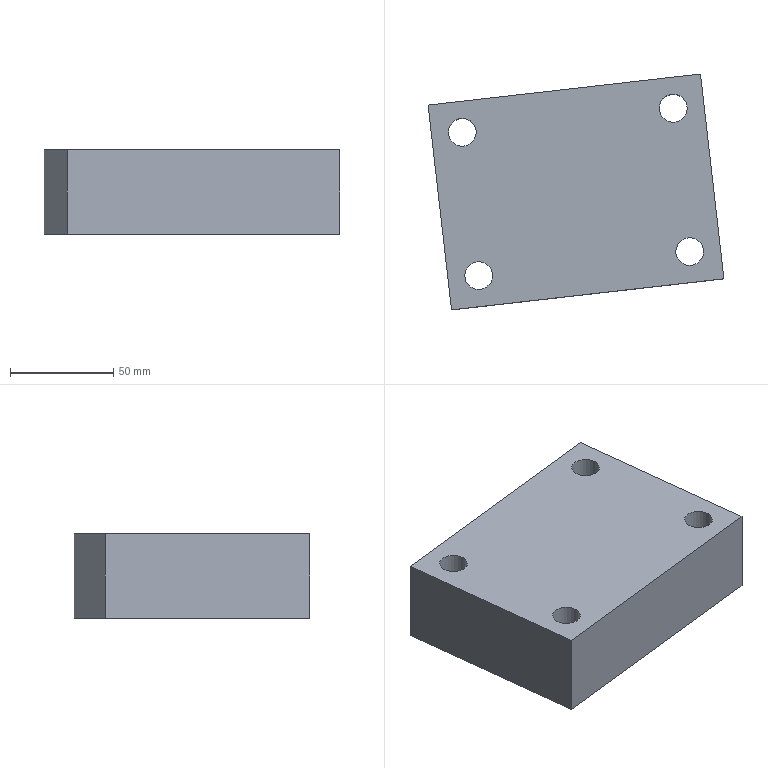Part | NX | features solid 2 | 1 solid | 18 faces | box 143.465 x 114.413 x 41 mm | volume 511564 mm3 | plane 10 | cylinder 8 | commonest cylinder face diameters 13.5 x4 20 x4
STEP:
#1=CARTESIAN_POINT('',(2599.823,120.761,101.));
#2=VERTEX_POINT('',#1);
#3=CARTESIAN_POINT('',(2593.073,120.761,101.));
#4=DIRECTION('',(0.,0.,1.));
#5=DIRECTION('',(1.,0.,0.));
#6=AXIS2_PLACEMENT_3D('',#3,#4,#5);
#7=CIRCLE('',#6,6.75);
#8=EDGE_CURVE('',#2,#2,#7,.T.);
#9=ORIENTED_EDGE('',*,*,#8,.F.);
#10=EDGE_LOOP('',(#9));
#11=FACE_BOUND('',#10,.T.);
#12=CARTESIAN_POINT('',(2607.575,52.73,101.));
#13=VERTEX_POINT('',#12);
#14=CARTESIAN_POINT('',(2600.998,51.211,101.));
#15=DIRECTION('',(0.,0.,-1.));
#16=DIRECTION('',(0.9744,0.225,0.));
#17=AXIS2_PLACEMENT_3D('',#14,#15,#16);
#18=CIRCLE('',#17,6.75);
#19=EDGE_CURVE('',#13,#13,#18,.T.);
#20=ORIENTED_EDGE('',*,*,#19,.T.);
#21=EDGE_LOOP('',(#20));
#22=FACE_BOUND('',#21,.T.);
#23=CARTESIAN_POINT('',(2606.279,137.363,101.));
#24=VERTEX_POINT('',#23);
#25=CARTESIAN_POINT('',(2474.134,122.307,101.));
#26=VERTEX_POINT('',#25);
#27=CARTESIAN_POINT('',(2529.774,128.646,101.));
#28=DIRECTION('',(-0.9936,-0.1132,0.));
#29=VECTOR('',#28,1000.);
#30=LINE('',#27,#29);
#31=EDGE_CURVE('',#24,#26,#30,.T.);
#32=ORIENTED_EDGE('',*,*,#31,.T.);
#33=CARTESIAN_POINT('',(2485.454,22.95,101.));
#34=VERTEX_POINT('',#33);
#35=CARTESIAN_POINT('',(2480.36,67.661,101.));
#36=DIRECTION('',(0.1132,-0.9936,0.));
#37=VECTOR('',#36,1000.);
#38=LINE('',#35,#37);
#39=EDGE_CURVE('',#26,#34,#38,.T.);
#40=ORIENTED_EDGE('',*,*,#39,.T.);
#41=CARTESIAN_POINT('',(2617.599,38.006,101.));
#42=VERTEX_POINT('',#41);
#43=CARTESIAN_POINT('',(2541.094,29.289,101.));
#44=DIRECTION('',(0.9936,0.1132,0.));
#45=VECTOR('',#44,1000.);
#46=LINE('',#43,#45);
#47=EDGE_CURVE('',#34,#42,#46,.T.);
#48=ORIENTED_EDGE('',*,*,#47,.T.);
#49=CARTESIAN_POINT('',(2612.505,82.717,101.));
#50=DIRECTION('',(-0.1132,0.9936,0.));
#51=VECTOR('',#50,1000.);
#52=LINE('',#49,#51);
#53=EDGE_CURVE('',#42,#24,#52,.T.);
#54=ORIENTED_EDGE('',*,*,#53,.T.);
#55=EDGE_LOOP('',(#32,#40,#48,#54));
#56=FACE_BOUND('',#55,.T.);
#57=CARTESIAN_POINT('',(2484.158,107.583,101.));
#58=VERTEX_POINT('',#57);
#59=CARTESIAN_POINT('',(2490.735,109.102,101.));
#60=DIRECTION('',(0.,0.,-1.));
#61=DIRECTION('',(-0.9744,-0.225,0.));
#62=AXIS2_PLACEMENT_3D('',#59,#60,#61);
#63=CIRCLE('',#62,6.75);
#64=EDGE_CURVE('',#58,#58,#63,.T.);
#65=ORIENTED_EDGE('',*,*,#64,.T.);
#66=EDGE_LOOP('',(#65));
#67=FACE_BOUND('',#66,.T.);
#68=CARTESIAN_POINT('',(2491.91,39.552,101.));
#69=VERTEX_POINT('',#68);
#70=CARTESIAN_POINT('',(2498.66,39.552,101.));
#71=DIRECTION('',(0.,0.,1.));
#72=DIRECTION('',(-1.,0.,0.));
#73=AXIS2_PLACEMENT_3D('',#70,#71,#72);
#74=CIRCLE('',#73,6.75);
#75=EDGE_CURVE('',#69,#69,#74,.T.);
#76=ORIENTED_EDGE('',*,*,#75,.F.);
#77=EDGE_LOOP('',(#76));
#78=FACE_BOUND('',#77,.T.);
#79=CARTESIAN_POINT('',(282.5,-193.,101.));
#80=DIRECTION('',(0.,0.,1.));
#81=DIRECTION('',(-1.,0.,0.));
#82=AXIS2_PLACEMENT_3D('',#79,#80,#81);
#83=PLANE('',#82);
#84=ADVANCED_FACE('',(#11,#22,#56,#67,#78),#83,.T.);
#85=CARTESIAN_POINT('',(2603.073,120.761,60.));
#86=VERTEX_POINT('',#85);
#87=CARTESIAN_POINT('',(2593.073,120.761,60.));
#88=DIRECTION('',(0.,0.,-1.));
#89=DIRECTION('',(1.,0.,0.));
#90=AXIS2_PLACEMENT_3D('',#87,#88,#89);
#91=CIRCLE('',#90,10.);
#92=EDGE_CURVE('',#86,#86,#91,.T.);
#93=ORIENTED_EDGE('',*,*,#92,.F.);
#94=EDGE_LOOP('',(#93));
#95=FACE_BOUND('',#94,.T.);
#96=CARTESIAN_POINT('',(2610.741,53.461,60.));
#97=VERTEX_POINT('',#96);
#98=CARTESIAN_POINT('',(2600.998,51.211,60.));
#99=DIRECTION('',(0.,0.,1.));
#100=DIRECTION('',(0.9744,0.225,0.));
#101=AXIS2_PLACEMENT_3D('',#98,#99,#100);
#102=CIRCLE('',#101,10.);
#103=EDGE_CURVE('',#97,#97,#102,.T.);
#104=ORIENTED_EDGE('',*,*,#103,.T.);
#105=EDGE_LOOP('',(#104));
#106=FACE_BOUND('',#105,.T.);
#107=CARTESIAN_POINT('',(2606.279,137.363,60.));
#108=VERTEX_POINT('',#107);
#109=CARTESIAN_POINT('',(2617.599,38.006,60.));
#110=VERTEX_POINT('',#109);
#111=CARTESIAN_POINT('',(2612.505,82.717,60.));
#112=DIRECTION('',(0.1132,-0.9936,0.));
#113=VECTOR('',#112,1000.);
#114=LINE('',#111,#113);
#115=EDGE_CURVE('',#108,#110,#114,.T.);
#116=ORIENTED_EDGE('',*,*,#115,.T.);
#117=CARTESIAN_POINT('',(2485.454,22.95,60.));
#118=VERTEX_POINT('',#117);
#119=CARTESIAN_POINT('',(2541.094,29.289,60.));
#120=DIRECTION('',(-0.9936,-0.1132,0.));
#121=VECTOR('',#120,1000.);
#122=LINE('',#119,#121);
#123=EDGE_CURVE('',#110,#118,#122,.T.);
#124=ORIENTED_EDGE('',*,*,#123,.T.);
#125=CARTESIAN_POINT('',(2474.134,122.307,60.));
#126=VERTEX_POINT('',#125);
#127=CARTESIAN_POINT('',(2480.36,67.661,60.));
#128=DIRECTION('',(-0.1132,0.9936,0.));
#129=VECTOR('',#128,1000.);
#130=LINE('',#127,#129);
#131=EDGE_CURVE('',#118,#126,#130,.T.);
#132=ORIENTED_EDGE('',*,*,#131,.T.);
#133=CARTESIAN_POINT('',(2529.774,128.646,60.));
#134=DIRECTION('',(0.9936,0.1132,0.));
#135=VECTOR('',#134,1000.);
#136=LINE('',#133,#135);
#137=EDGE_CURVE('',#126,#108,#136,.T.);
#138=ORIENTED_EDGE('',*,*,#137,.T.);
#139=EDGE_LOOP('',(#116,#124,#132,#138));
#140=FACE_BOUND('',#139,.T.);
#141=CARTESIAN_POINT('',(2480.992,106.852,60.));
#142=VERTEX_POINT('',#141);
#143=CARTESIAN_POINT('',(2490.735,109.102,60.));
#144=DIRECTION('',(0.,0.,1.));
#145=DIRECTION('',(-0.9744,-0.225,0.));
#146=AXIS2_PLACEMENT_3D('',#143,#144,#145);
#147=CIRCLE('',#146,10.);
#148=EDGE_CURVE('',#142,#142,#147,.T.);
#149=ORIENTED_EDGE('',*,*,#148,.T.);
#150=EDGE_LOOP('',(#149));
#151=FACE_BOUND('',#150,.T.);
#152=CARTESIAN_POINT('',(2488.66,39.552,60.));
#153=VERTEX_POINT('',#152);
#154=CARTESIAN_POINT('',(2498.66,39.552,60.));
#155=DIRECTION('',(0.,0.,-1.));
#156=DIRECTION('',(-1.,0.,0.));
#157=AXIS2_PLACEMENT_3D('',#154,#155,#156);
#158=CIRCLE('',#157,10.);
#159=EDGE_CURVE('',#153,#153,#158,.T.);
#160=ORIENTED_EDGE('',*,*,#159,.F.);
#161=EDGE_LOOP('',(#160));
#162=FACE_BOUND('',#161,.T.);
#163=CARTESIAN_POINT('',(2658.641,285.511,60.));
#164=DIRECTION('',(0.,0.,1.));
#165=DIRECTION('',(-1.,0.,0.));
#166=AXIS2_PLACEMENT_3D('',#163,#164,#165);
#167=PLANE('',#166);
#168=ADVANCED_FACE('',(#95,#106,#140,#151,#162),#167,.F.);
#169=CARTESIAN_POINT('',(2606.279,137.363,-10.));
#170=DIRECTION('',(0.,0.,1.));
#171=VECTOR('',#170,1000.);
#172=LINE('',#169,#171);
#173=EDGE_CURVE('',#108,#24,#172,.T.);
#174=ORIENTED_EDGE('',*,*,#173,.F.);
#175=ORIENTED_EDGE('',*,*,#137,.F.);
#176=CARTESIAN_POINT('',(2474.134,122.307,-10.));
#177=DIRECTION('',(0.,0.,1.));
#178=VECTOR('',#177,1000.);
#179=LINE('',#176,#178);
#180=EDGE_CURVE('',#126,#26,#179,.T.);
#181=ORIENTED_EDGE('',*,*,#180,.T.);
#182=ORIENTED_EDGE('',*,*,#31,.F.);
#183=EDGE_LOOP('',(#174,#175,#181,#182));
#184=FACE_BOUND('',#183,.T.);
#185=CARTESIAN_POINT('',(2529.774,128.646,-10.));
#186=DIRECTION('',(-0.1132,0.9936,0.));
#187=DIRECTION('',(-0.9936,-0.1132,0.));
#188=AXIS2_PLACEMENT_3D('',#185,#186,#187);
#189=PLANE('',#188);
#190=ADVANCED_FACE('',(#184),#189,.T.);
#191=ORIENTED_EDGE('',*,*,#180,.F.);
#192=ORIENTED_EDGE('',*,*,#131,.F.);
#193=CARTESIAN_POINT('',(2485.454,22.95,-10.));
#194=DIRECTION('',(0.,0.,1.));
#195=VECTOR('',#194,1000.);
#196=LINE('',#193,#195);
#197=EDGE_CURVE('',#118,#34,#196,.T.);
#198=ORIENTED_EDGE('',*,*,#197,.T.);
#199=ORIENTED_EDGE('',*,*,#39,.F.);
#200=EDGE_LOOP('',(#191,#192,#198,#199));
#201=FACE_BOUND('',#200,.T.);
#202=CARTESIAN_POINT('',(2480.36,67.661,-10.));
#203=DIRECTION('',(-0.9936,-0.1132,0.));
#204=DIRECTION('',(0.1132,-0.9936,0.));
#205=AXIS2_PLACEMENT_3D('',#202,#203,#204);
#206=PLANE('',#205);
#207=ADVANCED_FACE('',(#201),#206,.T.);
#208=ORIENTED_EDGE('',*,*,#197,.F.);
#209=ORIENTED_EDGE('',*,*,#123,.F.);
#210=CARTESIAN_POINT('',(2617.599,38.006,-10.));
#211=DIRECTION('',(0.,0.,1.));
#212=VECTOR('',#211,1000.);
#213=LINE('',#210,#212);
#214=EDGE_CURVE('',#110,#42,#213,.T.);
#215=ORIENTED_EDGE('',*,*,#214,.T.);
#216=ORIENTED_EDGE('',*,*,#47,.F.);
#217=EDGE_LOOP('',(#208,#209,#215,#216));
#218=FACE_BOUND('',#217,.T.);
#219=CARTESIAN_POINT('',(2541.094,29.289,-10.));
#220=DIRECTION('',(0.1132,-0.9936,0.));
#221=DIRECTION('',(0.9936,0.1132,0.));
#222=AXIS2_PLACEMENT_3D('',#219,#220,#221);
#223=PLANE('',#222);
#224=ADVANCED_FACE('',(#218),#223,.T.);
#225=ORIENTED_EDGE('',*,*,#115,.F.);
#226=ORIENTED_EDGE('',*,*,#173,.T.);
#227=ORIENTED_EDGE('',*,*,#53,.F.);
#228=ORIENTED_EDGE('',*,*,#214,.F.);
#229=EDGE_LOOP('',(#225,#226,#227,#228));
#230=FACE_BOUND('',#229,.T.);
#231=CARTESIAN_POINT('',(2612.505,82.717,-10.));
#232=DIRECTION('',(0.9936,0.1132,0.));
#233=DIRECTION('',(-0.1132,0.9936,0.));
#234=AXIS2_PLACEMENT_3D('',#231,#232,#233);
#235=PLANE('',#234);
#236=ADVANCED_FACE('',(#230),#235,.T.);
#237=CARTESIAN_POINT('',(2607.575,52.73,75.));
#238=VERTEX_POINT('',#237);
#239=CARTESIAN_POINT('',(2600.998,51.211,75.));
#240=DIRECTION('',(0.,0.,1.));
#241=DIRECTION('',(0.9744,0.225,0.));
#242=AXIS2_PLACEMENT_3D('',#239,#240,#241);
#243=CIRCLE('',#242,6.75);
#244=EDGE_CURVE('',#238,#238,#243,.T.);
#245=ORIENTED_EDGE('',*,*,#244,.F.);
#246=EDGE_LOOP('',(#245));
#247=FACE_BOUND('',#246,.T.);
#248=ORIENTED_EDGE('',*,*,#19,.F.);
#249=EDGE_LOOP('',(#248));
#250=FACE_BOUND('',#249,.T.);
#251=CARTESIAN_POINT('',(2600.998,51.211,60.));
#252=DIRECTION('',(0.,0.,1.));
#253=DIRECTION('',(-0.9744,-0.225,0.));
#254=AXIS2_PLACEMENT_3D('',#251,#252,#253);
#255=CYLINDRICAL_SURFACE('',#254,6.75);
#256=ADVANCED_FACE('',(#247,#250),#255,.F.);
#257=ORIENTED_EDGE('',*,*,#244,.T.);
#258=EDGE_LOOP('',(#257));
#259=FACE_BOUND('',#258,.T.);
#260=CARTESIAN_POINT('',(2610.741,53.461,75.));
#261=VERTEX_POINT('',#260);
#262=CARTESIAN_POINT('',(2600.998,51.211,75.));
#263=DIRECTION('',(0.,0.,1.));
#264=DIRECTION('',(0.9744,0.225,0.));
#265=AXIS2_PLACEMENT_3D('',#262,#263,#264);
#266=CIRCLE('',#265,10.);
#267=EDGE_CURVE('',#261,#261,#266,.T.);
#268=ORIENTED_EDGE('',*,*,#267,.F.);
#269=EDGE_LOOP('',(#268));
#270=FACE_BOUND('',#269,.T.);
#271=CARTESIAN_POINT('',(2600.998,51.211,75.));
#272=DIRECTION('',(0.,0.,1.));
#273=DIRECTION('',(-0.9744,-0.225,0.));
#274=AXIS2_PLACEMENT_3D('',#271,#272,#273);
#275=PLANE('',#274);
#276=ADVANCED_FACE('',(#259,#270),#275,.F.);
#277=ORIENTED_EDGE('',*,*,#267,.T.);
#278=EDGE_LOOP('',(#277));
#279=FACE_BOUND('',#278,.T.);
#280=ORIENTED_EDGE('',*,*,#103,.F.);
#281=EDGE_LOOP('',(#280));
#282=FACE_BOUND('',#281,.T.);
#283=CARTESIAN_POINT('',(2600.998,51.211,60.));
#284=DIRECTION('',(0.,0.,1.));
#285=DIRECTION('',(-0.9744,-0.225,0.));
#286=AXIS2_PLACEMENT_3D('',#283,#284,#285);
#287=CYLINDRICAL_SURFACE('',#286,10.);
#288=ADVANCED_FACE('',(#279,#282),#287,.F.);
#289=CARTESIAN_POINT('',(2599.823,120.761,75.));
#290=VERTEX_POINT('',#289);
#291=CARTESIAN_POINT('',(2593.073,120.761,75.));
#292=DIRECTION('',(0.,0.,-1.));
#293=DIRECTION('',(1.,0.,0.));
#294=AXIS2_PLACEMENT_3D('',#291,#292,#293);
#295=CIRCLE('',#294,6.75);
#296=EDGE_CURVE('',#290,#290,#295,.T.);
#297=ORIENTED_EDGE('',*,*,#296,.T.);
#298=EDGE_LOOP('',(#297));
#299=FACE_BOUND('',#298,.T.);
#300=ORIENTED_EDGE('',*,*,#8,.T.);
#301=EDGE_LOOP('',(#300));
#302=FACE_BOUND('',#301,.T.);
#303=CARTESIAN_POINT('',(2593.073,120.761,60.));
#304=DIRECTION('',(0.,0.,1.));
#305=DIRECTION('',(-1.,0.,0.));
#306=AXIS2_PLACEMENT_3D('',#303,#304,#305);
#307=CYLINDRICAL_SURFACE('',#306,6.75);
#308=ADVANCED_FACE('',(#299,#302),#307,.F.);
#309=ORIENTED_EDGE('',*,*,#296,.F.);
#310=EDGE_LOOP('',(#309));
#311=FACE_BOUND('',#310,.T.);
#312=CARTESIAN_POINT('',(2603.073,120.761,75.));
#313=VERTEX_POINT('',#312);
#314=CARTESIAN_POINT('',(2593.073,120.761,75.));
#315=DIRECTION('',(0.,0.,-1.));
#316=DIRECTION('',(1.,0.,0.));
#317=AXIS2_PLACEMENT_3D('',#314,#315,#316);
#318=CIRCLE('',#317,10.);
#319=EDGE_CURVE('',#313,#313,#318,.T.);
#320=ORIENTED_EDGE('',*,*,#319,.T.);
#321=EDGE_LOOP('',(#320));
#322=FACE_BOUND('',#321,.T.);
#323=CARTESIAN_POINT('',(2593.073,120.761,75.));
#324=DIRECTION('',(0.,0.,1.));
#325=DIRECTION('',(-1.,0.,0.));
#326=AXIS2_PLACEMENT_3D('',#323,#324,#325);
#327=PLANE('',#326);
#328=ADVANCED_FACE('',(#311,#322),#327,.F.);
#329=ORIENTED_EDGE('',*,*,#319,.F.);
#330=EDGE_LOOP('',(#329));
#331=FACE_BOUND('',#330,.T.);
#332=ORIENTED_EDGE('',*,*,#92,.T.);
#333=EDGE_LOOP('',(#332));
#334=FACE_BOUND('',#333,.T.);
#335=CARTESIAN_POINT('',(2593.073,120.761,60.));
#336=DIRECTION('',(0.,0.,1.));
#337=DIRECTION('',(-1.,0.,0.));
#338=AXIS2_PLACEMENT_3D('',#335,#336,#337);
#339=CYLINDRICAL_SURFACE('',#338,10.);
#340=ADVANCED_FACE('',(#331,#334),#339,.F.);
#341=CARTESIAN_POINT('',(2484.158,107.583,75.));
#342=VERTEX_POINT('',#341);
#343=CARTESIAN_POINT('',(2490.735,109.102,75.));
#344=DIRECTION('',(0.,0.,1.));
#345=DIRECTION('',(-0.9744,-0.225,0.));
#346=AXIS2_PLACEMENT_3D('',#343,#344,#345);
#347=CIRCLE('',#346,6.75);
#348=EDGE_CURVE('',#342,#342,#347,.T.);
#349=ORIENTED_EDGE('',*,*,#348,.F.);
#350=EDGE_LOOP('',(#349));
#351=FACE_BOUND('',#350,.T.);
#352=ORIENTED_EDGE('',*,*,#64,.F.);
#353=EDGE_LOOP('',(#352));
#354=FACE_BOUND('',#353,.T.);
#355=CARTESIAN_POINT('',(2490.735,109.102,60.));
#356=DIRECTION('',(0.,0.,1.));
#357=DIRECTION('',(0.9744,0.225,0.));
#358=AXIS2_PLACEMENT_3D('',#355,#356,#357);
#359=CYLINDRICAL_SURFACE('',#358,6.75);
#360=ADVANCED_FACE('',(#351,#354),#359,.F.);
#361=ORIENTED_EDGE('',*,*,#348,.T.);
#362=EDGE_LOOP('',(#361));
#363=FACE_BOUND('',#362,.T.);
#364=CARTESIAN_POINT('',(2480.992,106.852,75.));
#365=VERTEX_POINT('',#364);
#366=CARTESIAN_POINT('',(2490.735,109.102,75.));
#367=DIRECTION('',(0.,0.,1.));
#368=DIRECTION('',(-0.9744,-0.225,0.));
#369=AXIS2_PLACEMENT_3D('',#366,#367,#368);
#370=CIRCLE('',#369,10.);
#371=EDGE_CURVE('',#365,#365,#370,.T.);
#372=ORIENTED_EDGE('',*,*,#371,.F.);
#373=EDGE_LOOP('',(#372));
#374=FACE_BOUND('',#373,.T.);
#375=CARTESIAN_POINT('',(2490.735,109.102,75.));
#376=DIRECTION('',(0.,0.,1.));
#377=DIRECTION('',(0.9744,0.225,0.));
#378=AXIS2_PLACEMENT_3D('',#375,#376,#377);
#379=PLANE('',#378);
#380=ADVANCED_FACE('',(#363,#374),#379,.F.);
#381=ORIENTED_EDGE('',*,*,#371,.T.);
#382=EDGE_LOOP('',(#381));
#383=FACE_BOUND('',#382,.T.);
#384=ORIENTED_EDGE('',*,*,#148,.F.);
#385=EDGE_LOOP('',(#384));
#386=FACE_BOUND('',#385,.T.);
#387=CARTESIAN_POINT('',(2490.735,109.102,60.));
#388=DIRECTION('',(0.,0.,1.));
#389=DIRECTION('',(0.9744,0.225,0.));
#390=AXIS2_PLACEMENT_3D('',#387,#388,#389);
#391=CYLINDRICAL_SURFACE('',#390,10.);
#392=ADVANCED_FACE('',(#383,#386),#391,.F.);
#393=CARTESIAN_POINT('',(2491.91,39.552,75.));
#394=VERTEX_POINT('',#393);
#395=CARTESIAN_POINT('',(2498.66,39.552,75.));
#396=DIRECTION('',(0.,0.,-1.));
#397=DIRECTION('',(-1.,0.,0.));
#398=AXIS2_PLACEMENT_3D('',#395,#396,#397);
#399=CIRCLE('',#398,6.75);
#400=EDGE_CURVE('',#394,#394,#399,.T.);
#401=ORIENTED_EDGE('',*,*,#400,.T.);
#402=EDGE_LOOP('',(#401));
#403=FACE_BOUND('',#402,.T.);
#404=ORIENTED_EDGE('',*,*,#75,.T.);
#405=EDGE_LOOP('',(#404));
#406=FACE_BOUND('',#405,.T.);
#407=CARTESIAN_POINT('',(2498.66,39.552,60.));
#408=DIRECTION('',(0.,0.,1.));
#409=DIRECTION('',(1.,0.,0.));
#410=AXIS2_PLACEMENT_3D('',#407,#408,#409);
#411=CYLINDRICAL_SURFACE('',#410,6.75);
#412=ADVANCED_FACE('',(#403,#406),#411,.F.);
#413=ORIENTED_EDGE('',*,*,#400,.F.);
#414=EDGE_LOOP('',(#413));
#415=FACE_BOUND('',#414,.T.);
#416=CARTESIAN_POINT('',(2488.66,39.552,75.));
#417=VERTEX_POINT('',#416);
#418=CARTESIAN_POINT('',(2498.66,39.552,75.));
#419=DIRECTION('',(0.,0.,-1.));
#420=DIRECTION('',(-1.,0.,0.));
#421=AXIS2_PLACEMENT_3D('',#418,#419,#420);
#422=CIRCLE('',#421,10.);
#423=EDGE_CURVE('',#417,#417,#422,.T.);
#424=ORIENTED_EDGE('',*,*,#423,.T.);
#425=EDGE_LOOP('',(#424));
#426=FACE_BOUND('',#425,.T.);
#427=CARTESIAN_POINT('',(2498.66,39.552,75.));
#428=DIRECTION('',(0.,0.,1.));
#429=DIRECTION('',(1.,0.,0.));
#430=AXIS2_PLACEMENT_3D('',#427,#428,#429);
#431=PLANE('',#430);
#432=ADVANCED_FACE('',(#415,#426),#431,.F.);
#433=ORIENTED_EDGE('',*,*,#423,.F.);
#434=EDGE_LOOP('',(#433));
#435=FACE_BOUND('',#434,.T.);
#436=ORIENTED_EDGE('',*,*,#159,.T.);
#437=EDGE_LOOP('',(#436));
#438=FACE_BOUND('',#437,.T.);
#439=CARTESIAN_POINT('',(2498.66,39.552,60.));
#440=DIRECTION('',(0.,0.,1.));
#441=DIRECTION('',(1.,0.,0.));
#442=AXIS2_PLACEMENT_3D('',#439,#440,#441);
#443=CYLINDRICAL_SURFACE('',#442,10.);
#444=ADVANCED_FACE('',(#435,#438),#443,.F.);
#445=CLOSED_SHELL('',(#84,#168,#190,#207,#224,#236,#256,#276,#288,#308,#328,#340,#360,#380,#392,#412,#432,#444));
#446=MANIFOLD_SOLID_BREP('',#445);
#447=(LENGTH_UNIT()NAMED_UNIT(*)SI_UNIT(.MILLI.,.METRE.));
#448=UNCERTAINTY_MEASURE_WITH_UNIT(LENGTH_MEASURE(0.00001),#447,'','');
#449=(NAMED_UNIT(*)PLANE_ANGLE_UNIT()SI_UNIT($,.RADIAN.));
#450=(NAMED_UNIT(*)SI_UNIT($,.STERADIAN.)SOLID_ANGLE_UNIT());
#451=(GEOMETRIC_REPRESENTATION_CONTEXT(3)GLOBAL_UNCERTAINTY_ASSIGNED_CONTEXT((#448))GLOBAL_UNIT_ASSIGNED_CONTEXT((#447,#449,#450))REPRESENTATION_CONTEXT('',''));
#452=ADVANCED_BREP_SHAPE_REPRESENTATION('',(#446),#451);